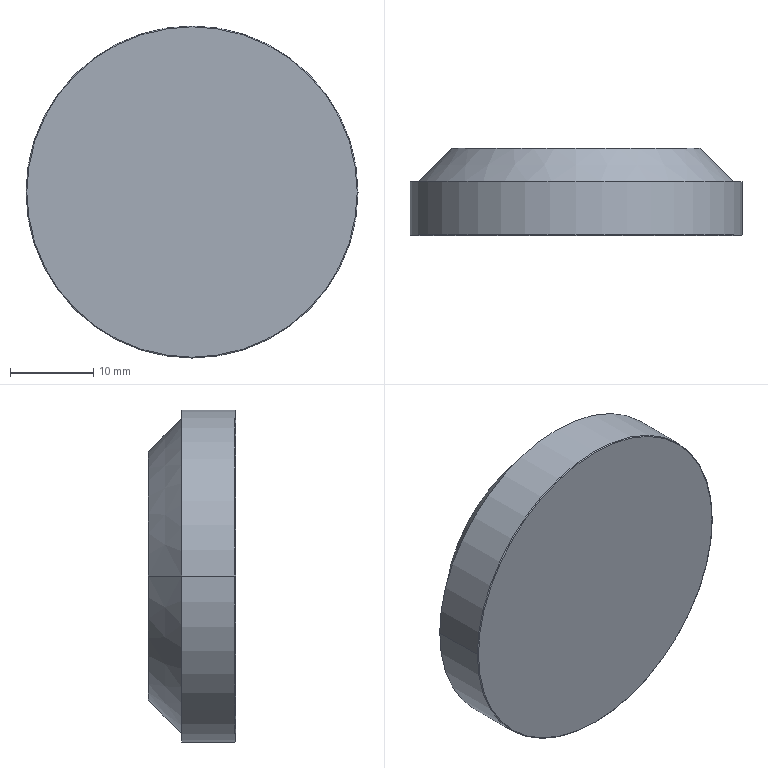Part | NX | 1 solid | 9 faces | box 40 x 10.5 x 40 mm | volume 11816 mm3 | plane 3 | torus 2 | cylinder 2 | cone 2 | commonest cylinder face diameters 40 x2
STEP:
#1=CARTESIAN_POINT('',(-19.9,0.,0.));
#2=VERTEX_POINT('',#1);
#3=CARTESIAN_POINT('',(19.9,0.,0.));
#4=VERTEX_POINT('',#3);
#5=CARTESIAN_POINT('',(0.,0.,0.));
#6=DIRECTION('',(0.,1.,0.));
#7=DIRECTION('',(1.,0.,0.));
#8=AXIS2_PLACEMENT_3D('',#5,#6,#7);
#9=CIRCLE('',#8,19.9);
#10=EDGE_CURVE('',#2,#4,#9,.T.);
#11=ORIENTED_EDGE('',*,*,#10,.F.);
#12=CARTESIAN_POINT('',(0.,0.,0.));
#13=DIRECTION('',(0.,1.,0.));
#14=DIRECTION('',(1.,0.,0.));
#15=AXIS2_PLACEMENT_3D('',#12,#13,#14);
#16=CIRCLE('',#15,19.9);
#17=EDGE_CURVE('',#4,#2,#16,.T.);
#18=ORIENTED_EDGE('',*,*,#17,.F.);
#19=EDGE_LOOP('',(#11,#18));
#20=FACE_BOUND('',#19,.T.);
#21=CARTESIAN_POINT('',(0.,0.,0.));
#22=DIRECTION('',(0.,-1.,0.));
#23=DIRECTION('',(0.,0.,-1.));
#24=AXIS2_PLACEMENT_3D('',#21,#22,#23);
#25=PLANE('',#24);
#26=ADVANCED_FACE('',(#20),#25,.T.);
#27=CARTESIAN_POINT('',(-20.,0.1,0.));
#28=VERTEX_POINT('',#27);
#29=CARTESIAN_POINT('',(20.,0.1,0.));
#30=VERTEX_POINT('',#29);
#31=CARTESIAN_POINT('',(0.,0.1,0.));
#32=DIRECTION('',(0.,1.,0.));
#33=DIRECTION('',(-1.,0.,0.));
#34=AXIS2_PLACEMENT_3D('',#31,#32,#33);
#35=CIRCLE('',#34,20.);
#36=EDGE_CURVE('',#28,#30,#35,.T.);
#37=ORIENTED_EDGE('',*,*,#36,.F.);
#38=CARTESIAN_POINT('',(-19.9,0.1,0.));
#39=DIRECTION('',(0.,0.,-1.));
#40=DIRECTION('',(-1.,0.,0.));
#41=AXIS2_PLACEMENT_3D('',#38,#39,#40);
#42=CIRCLE('',#41,0.1);
#43=EDGE_CURVE('',#28,#2,#42,.F.);
#44=ORIENTED_EDGE('',*,*,#43,.T.);
#45=ORIENTED_EDGE('',*,*,#10,.T.);
#46=CARTESIAN_POINT('',(19.9,0.1,0.));
#47=DIRECTION('',(0.,0.,1.));
#48=DIRECTION('',(1.,0.,0.));
#49=AXIS2_PLACEMENT_3D('',#46,#47,#48);
#50=CIRCLE('',#49,0.1);
#51=EDGE_CURVE('',#30,#4,#50,.F.);
#52=ORIENTED_EDGE('',*,*,#51,.F.);
#53=EDGE_LOOP('',(#37,#44,#45,#52));
#54=FACE_BOUND('',#53,.T.);
#55=CARTESIAN_POINT('',(0.,0.1,0.));
#56=DIRECTION('',(0.,-1.,0.));
#57=DIRECTION('',(-1.,0.,0.));
#58=AXIS2_PLACEMENT_3D('',#55,#56,#57);
#59=TOROIDAL_SURFACE('',#58,19.9,0.1);
#60=ADVANCED_FACE('',(#54),#59,.T.);
#61=CARTESIAN_POINT('',(-15.,10.5,0.));
#62=VERTEX_POINT('',#61);
#63=CARTESIAN_POINT('',(15.,10.5,0.));
#64=VERTEX_POINT('',#63);
#65=CARTESIAN_POINT('',(0.,10.5,0.));
#66=DIRECTION('',(0.,-1.,0.));
#67=DIRECTION('',(1.,0.,0.));
#68=AXIS2_PLACEMENT_3D('',#65,#66,#67);
#69=CIRCLE('',#68,15.);
#70=EDGE_CURVE('',#62,#64,#69,.T.);
#71=ORIENTED_EDGE('',*,*,#70,.F.);
#72=CARTESIAN_POINT('',(0.,10.5,0.));
#73=DIRECTION('',(0.,-1.,0.));
#74=DIRECTION('',(1.,0.,0.));
#75=AXIS2_PLACEMENT_3D('',#72,#73,#74);
#76=CIRCLE('',#75,15.);
#77=EDGE_CURVE('',#64,#62,#76,.T.);
#78=ORIENTED_EDGE('',*,*,#77,.F.);
#79=EDGE_LOOP('',(#71,#78));
#80=FACE_BOUND('',#79,.T.);
#81=CARTESIAN_POINT('',(0.,10.5,0.));
#82=DIRECTION('',(0.,-1.,0.));
#83=DIRECTION('',(0.,0.,-1.));
#84=AXIS2_PLACEMENT_3D('',#81,#82,#83);
#85=PLANE('',#84);
#86=ADVANCED_FACE('',(#80),#85,.F.);
#87=CARTESIAN_POINT('',(-20.,6.5,0.));
#88=VERTEX_POINT('',#87);
#89=CARTESIAN_POINT('',(20.,6.5,0.));
#90=VERTEX_POINT('',#89);
#91=CARTESIAN_POINT('',(0.,6.5,0.));
#92=DIRECTION('',(0.,-1.,0.));
#93=DIRECTION('',(1.,0.,0.));
#94=AXIS2_PLACEMENT_3D('',#91,#92,#93);
#95=CIRCLE('',#94,20.);
#96=EDGE_CURVE('',#88,#90,#95,.T.);
#97=ORIENTED_EDGE('',*,*,#96,.T.);
#98=CARTESIAN_POINT('',(20.,11.025,0.));
#99=DIRECTION('',(0.,-1.,0.));
#100=VECTOR('',#99,1000.);
#101=LINE('',#98,#100);
#102=EDGE_CURVE('',#90,#30,#101,.T.);
#103=ORIENTED_EDGE('',*,*,#102,.T.);
#104=CARTESIAN_POINT('',(0.,0.1,0.));
#105=DIRECTION('',(0.,1.,0.));
#106=DIRECTION('',(-1.,0.,0.));
#107=AXIS2_PLACEMENT_3D('',#104,#105,#106);
#108=CIRCLE('',#107,20.);
#109=EDGE_CURVE('',#30,#28,#108,.T.);
#110=ORIENTED_EDGE('',*,*,#109,.T.);
#111=CARTESIAN_POINT('',(-20.,11.025,0.));
#112=DIRECTION('',(0.,-1.,0.));
#113=VECTOR('',#112,1000.);
#114=LINE('',#111,#113);
#115=EDGE_CURVE('',#88,#28,#114,.T.);
#116=ORIENTED_EDGE('',*,*,#115,.F.);
#117=EDGE_LOOP('',(#97,#103,#110,#116));
#118=FACE_BOUND('',#117,.T.);
#119=CARTESIAN_POINT('',(0.,11.025,0.));
#120=DIRECTION('',(0.,-1.,0.));
#121=DIRECTION('',(-1.,0.,0.));
#122=AXIS2_PLACEMENT_3D('',#119,#120,#121);
#123=CYLINDRICAL_SURFACE('',#122,20.);
#124=ADVANCED_FACE('',(#118),#123,.T.);
#125=ORIENTED_EDGE('',*,*,#70,.T.);
#126=CARTESIAN_POINT('',(19.,6.5,0.));
#127=VERTEX_POINT('',#126);
#128=CARTESIAN_POINT('',(17.,8.5,0.));
#129=DIRECTION('',(0.7071,-0.7071,0.));
#130=VECTOR('',#129,1000.);
#131=LINE('',#128,#130);
#132=EDGE_CURVE('',#127,#64,#131,.F.);
#133=ORIENTED_EDGE('',*,*,#132,.F.);
#134=CARTESIAN_POINT('',(-19.,6.5,0.));
#135=VERTEX_POINT('',#134);
#136=CARTESIAN_POINT('',(0.,6.5,0.));
#137=DIRECTION('',(0.,1.,0.));
#138=DIRECTION('',(1.,0.,0.));
#139=AXIS2_PLACEMENT_3D('',#136,#137,#138);
#140=CIRCLE('',#139,19.);
#141=EDGE_CURVE('',#127,#135,#140,.T.);
#142=ORIENTED_EDGE('',*,*,#141,.T.);
#143=CARTESIAN_POINT('',(-17.,8.5,0.));
#144=DIRECTION('',(-0.7071,-0.7071,0.));
#145=VECTOR('',#144,1000.);
#146=LINE('',#143,#145);
#147=EDGE_CURVE('',#135,#62,#146,.F.);
#148=ORIENTED_EDGE('',*,*,#147,.T.);
#149=EDGE_LOOP('',(#125,#133,#142,#148));
#150=FACE_BOUND('',#149,.T.);
#151=CARTESIAN_POINT('',(0.,8.5,0.));
#152=DIRECTION('',(0.,-1.,0.));
#153=DIRECTION('',(-1.,0.,0.));
#154=AXIS2_PLACEMENT_3D('',#151,#152,#153);
#155=CONICAL_SURFACE('',#154,17.,0.7854);
#156=ADVANCED_FACE('',(#150),#155,.T.);
#157=ORIENTED_EDGE('',*,*,#96,.F.);
#158=CARTESIAN_POINT('',(0.,6.5,0.));
#159=DIRECTION('',(0.,-1.,0.));
#160=DIRECTION('',(1.,0.,0.));
#161=AXIS2_PLACEMENT_3D('',#158,#159,#160);
#162=CIRCLE('',#161,20.);
#163=EDGE_CURVE('',#90,#88,#162,.T.);
#164=ORIENTED_EDGE('',*,*,#163,.F.);
#165=EDGE_LOOP('',(#157,#164));
#166=FACE_BOUND('',#165,.T.);
#167=ORIENTED_EDGE('',*,*,#141,.F.);
#168=CARTESIAN_POINT('',(0.,6.5,0.));
#169=DIRECTION('',(0.,1.,0.));
#170=DIRECTION('',(1.,0.,0.));
#171=AXIS2_PLACEMENT_3D('',#168,#169,#170);
#172=CIRCLE('',#171,19.);
#173=EDGE_CURVE('',#135,#127,#172,.T.);
#174=ORIENTED_EDGE('',*,*,#173,.F.);
#175=EDGE_LOOP('',(#167,#174));
#176=FACE_BOUND('',#175,.T.);
#177=CARTESIAN_POINT('',(0.,6.5,0.));
#178=DIRECTION('',(0.,-1.,0.));
#179=DIRECTION('',(0.,0.,-1.));
#180=AXIS2_PLACEMENT_3D('',#177,#178,#179);
#181=PLANE('',#180);
#182=ADVANCED_FACE('',(#166,#176),#181,.F.);
#183=ORIENTED_EDGE('',*,*,#36,.T.);
#184=ORIENTED_EDGE('',*,*,#102,.F.);
#185=ORIENTED_EDGE('',*,*,#163,.T.);
#186=ORIENTED_EDGE('',*,*,#115,.T.);
#187=EDGE_LOOP('',(#183,#184,#185,#186));
#188=FACE_BOUND('',#187,.T.);
#189=CARTESIAN_POINT('',(0.,11.025,0.));
#190=DIRECTION('',(0.,-1.,0.));
#191=DIRECTION('',(-1.,0.,0.));
#192=AXIS2_PLACEMENT_3D('',#189,#190,#191);
#193=CYLINDRICAL_SURFACE('',#192,20.);
#194=ADVANCED_FACE('',(#188),#193,.T.);
#195=ORIENTED_EDGE('',*,*,#147,.F.);
#196=ORIENTED_EDGE('',*,*,#173,.T.);
#197=ORIENTED_EDGE('',*,*,#132,.T.);
#198=ORIENTED_EDGE('',*,*,#77,.T.);
#199=EDGE_LOOP('',(#195,#196,#197,#198));
#200=FACE_BOUND('',#199,.T.);
#201=CARTESIAN_POINT('',(0.,8.5,0.));
#202=DIRECTION('',(0.,-1.,0.));
#203=DIRECTION('',(-1.,0.,0.));
#204=AXIS2_PLACEMENT_3D('',#201,#202,#203);
#205=CONICAL_SURFACE('',#204,17.,0.7854);
#206=ADVANCED_FACE('',(#200),#205,.T.);
#207=ORIENTED_EDGE('',*,*,#43,.F.);
#208=ORIENTED_EDGE('',*,*,#109,.F.);
#209=ORIENTED_EDGE('',*,*,#51,.T.);
#210=ORIENTED_EDGE('',*,*,#17,.T.);
#211=EDGE_LOOP('',(#207,#208,#209,#210));
#212=FACE_BOUND('',#211,.T.);
#213=CARTESIAN_POINT('',(0.,0.1,0.));
#214=DIRECTION('',(0.,-1.,0.));
#215=DIRECTION('',(-1.,0.,0.));
#216=AXIS2_PLACEMENT_3D('',#213,#214,#215);
#217=TOROIDAL_SURFACE('',#216,19.9,0.1);
#218=ADVANCED_FACE('',(#212),#217,.T.);
#219=CLOSED_SHELL('',(#26,#60,#86,#124,#156,#182,#194,#206,#218));
#220=MANIFOLD_SOLID_BREP('',#219);
#221=(LENGTH_UNIT()NAMED_UNIT(*)SI_UNIT(.MILLI.,.METRE.));
#222=UNCERTAINTY_MEASURE_WITH_UNIT(LENGTH_MEASURE(0.00001),#221,'','');
#223=(NAMED_UNIT(*)PLANE_ANGLE_UNIT()SI_UNIT($,.RADIAN.));
#224=(NAMED_UNIT(*)SI_UNIT($,.STERADIAN.)SOLID_ANGLE_UNIT());
#225=(GEOMETRIC_REPRESENTATION_CONTEXT(3)GLOBAL_UNCERTAINTY_ASSIGNED_CONTEXT((#222))GLOBAL_UNIT_ASSIGNED_CONTEXT((#221,#223,#224))REPRESENTATION_CONTEXT('',''));
#226=ADVANCED_BREP_SHAPE_REPRESENTATION('',(#220),#225);